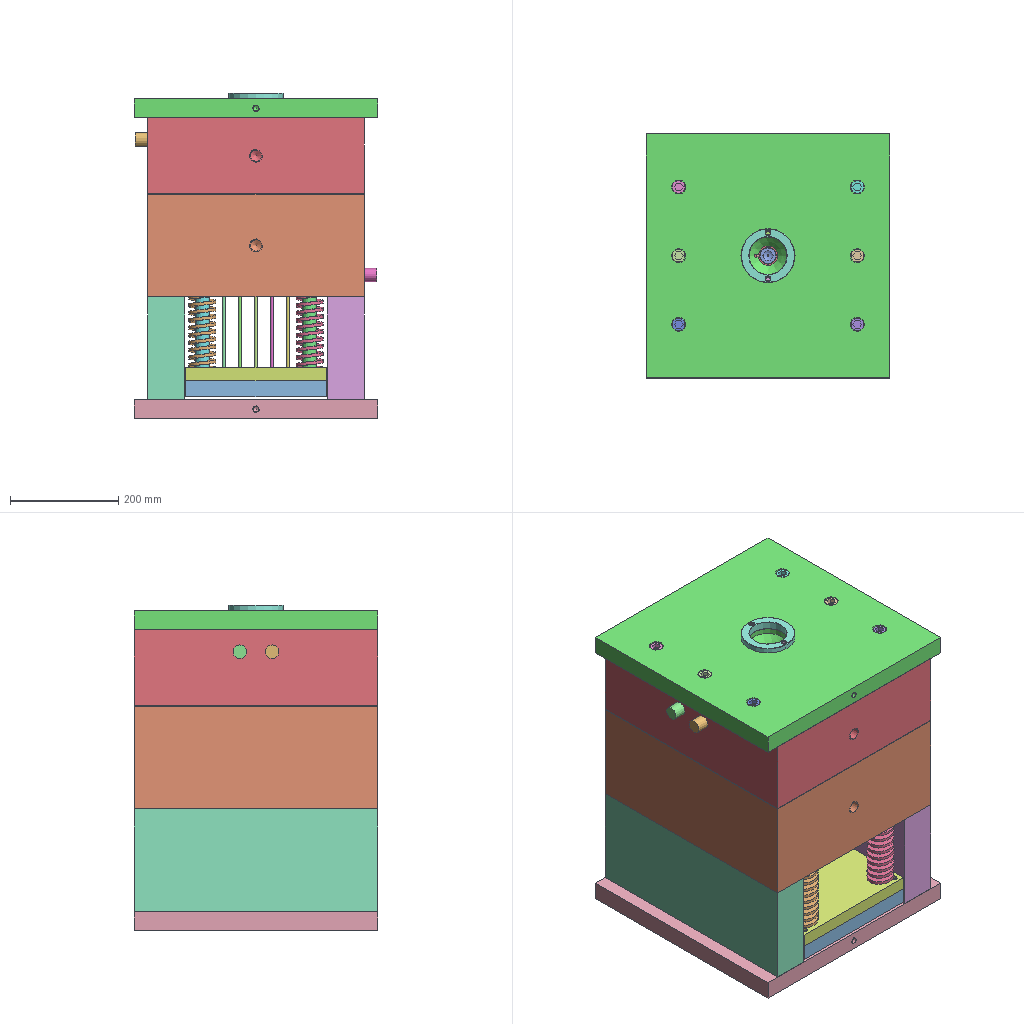Assembly | NX | 144 different items | 144 placed | box 450 x 450 x 601 mm
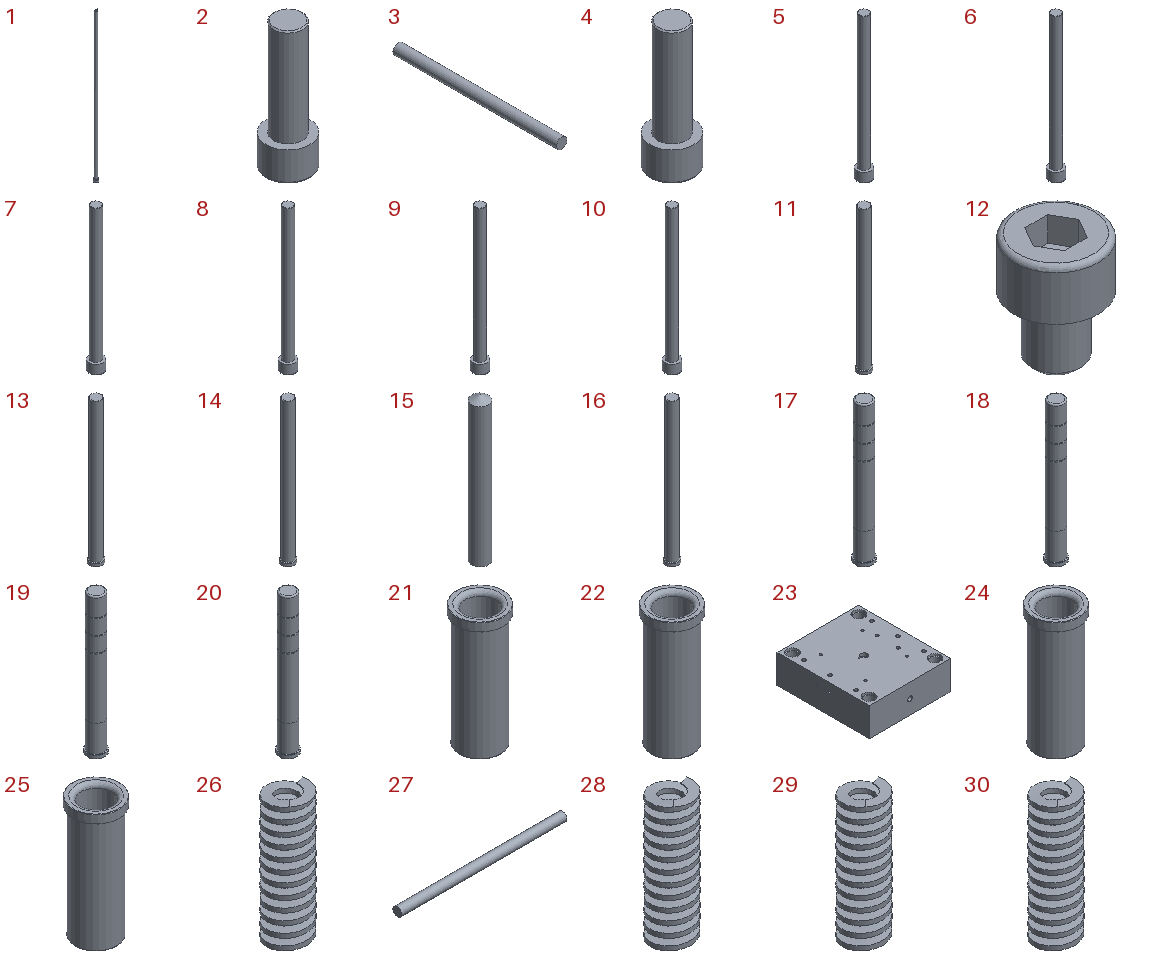Parts list (item | quantity | size | volume | features):
1 | x1 | 10 x 10 x 360.85 mm | 10434 mm3 | features solid 2
2 | x1 | 18 x 18 x 52 mm | 7050 mm3 | features solid 2
3 | x1 | 6 x 95.732 x 6 mm | 2674 mm3 | features solid 2
4 | x1 | 18 x 18 x 52 mm | 7050 mm3 | features solid 2
5 | x1 | 24 x 24 x 246 mm | 52114 mm3 | features solid 2
6 | x1 | 24 x 24 x 246 mm | 52114 mm3 | features solid 2
7 | x1 | 24 x 24 x 246 mm | 52114 mm3 | features solid 2
8 | x1 | 24 x 24 x 246 mm | 52114 mm3 | features solid 2
9 | x1 | 24 x 24 x 246 mm | 52114 mm3 | features solid 2
10 | x1 | 24 x 24 x 246 mm | 52114 mm3 | features solid 2
11 | x1 | 30 x 30 x 346 mm | 171537 mm3 | features solid 2
12 | x1 | 8.5 x 8.5 x 11 mm | 363.666 mm3 | features solid 2
13 | x1 | 30 x 30 x 346 mm | 171537 mm3 | features solid 2
14 | x1 | 30 x 30 x 346 mm | 171537 mm3 | features solid 2
15 | x1 | 6 x 6 x 50.732 mm | 1402 mm3 | features solid 2
16 | x1 | 30 x 30 x 346 mm | 171537 mm3 | features solid 2
17 | x1 | 40 x 40 x 320 mm | 309816 mm3 | features solid 2
18 | x1 | 40 x 40 x 320 mm | 309816 mm3 | features solid 2
19 | x1 | 40 x 40 x 320 mm | 309816 mm3 | features solid 2
20 | x1 | 40 x 40 x 320 mm | 309816 mm3 | features solid 2
21 | x1 | 54 x 54 x 140 mm | 122133 mm3 | features solid 2
22 | x1 | 54 x 54 x 140 mm | 122133 mm3 | features solid 2
23 | x1 | 400 x 450 x 140 mm | 19391135 mm3 | features solid 2
24 | x1 | 54 x 54 x 140 mm | 122133 mm3 | features solid 2
25 | x1 | 54 x 54 x 140 mm | 122133 mm3 | features solid 2
26 | x1 | 50.009 x 50.008 x 160 mm | 82264 mm3 | features solid 2
27 | x1 | 115 x 6 x 6 mm | 3252 mm3 | features solid 2
28 | x1 | 50.009 x 50.008 x 160 mm | 82264 mm3 | features solid 2
29 | x1 | 50.009 x 50.008 x 160 mm | 82264 mm3 | features solid 2
30 | x1 | 50.009 x 50.008 x 160 mm | 82264 mm3 | features solid 2
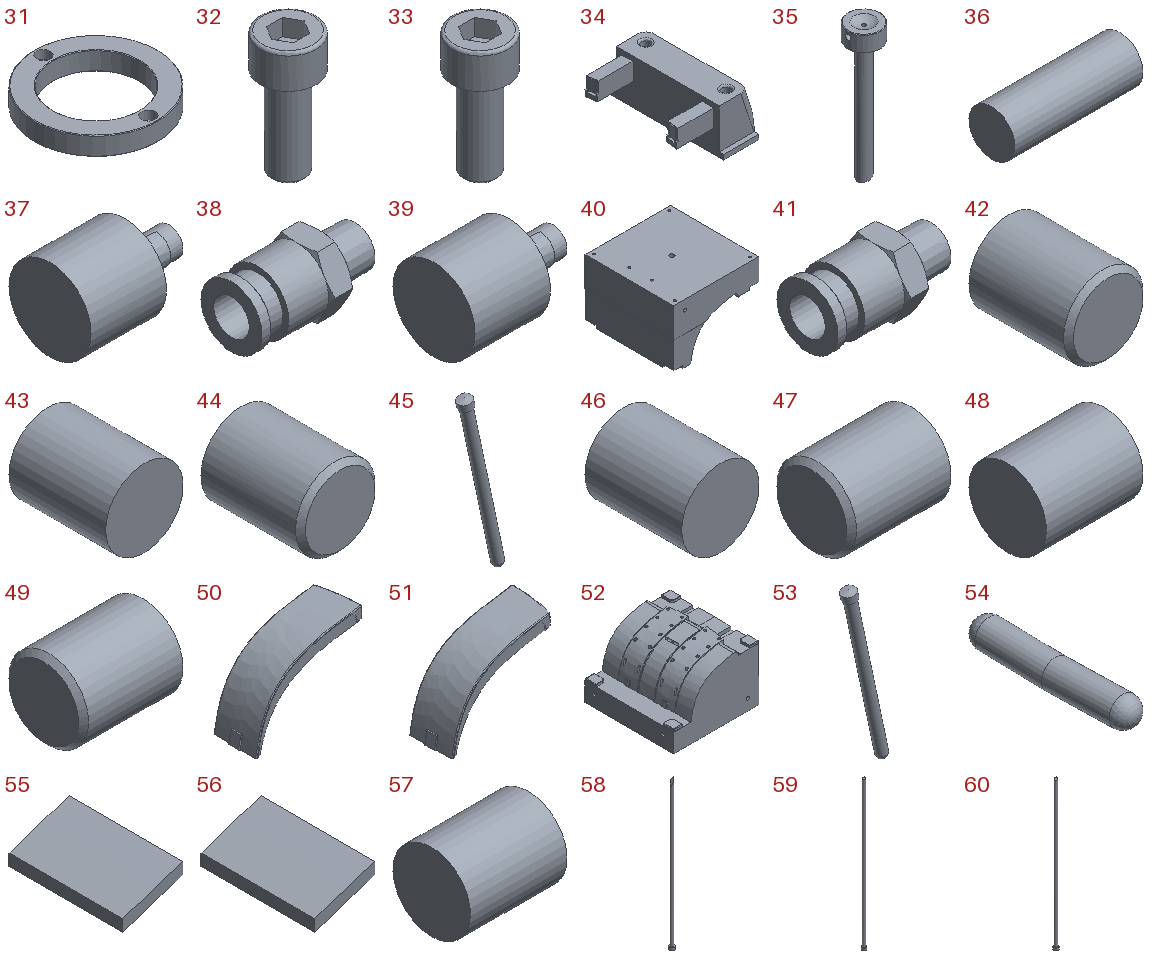31 | x1 | 99.8 x 99.8 x 15 mm | 57533 mm3 | features solid 2
32 | x1 | 10 x 10 x 22 mm | 854.803 mm3 | features solid 2
33 | x1 | 10 x 10 x 22 mm | 854.803 mm3 | features solid 2
34 | x1 | 92.291 x 144 x 57 mm | 348793 mm3 | features solid 2
35 | x1 | 30 x 30 x 126.717 mm | 19254 mm3 | features solid 2
36 | x1 | 14 x 5 x 5 mm | 274.889 mm3 | features solid 2
37 | x1 | 38.754 x 25 x 25 mm | 12122 mm3 | features solid 2
38 | x1 | 27.9 x 16.166 x 14 mm | 2279 mm3 | features solid 2
39 | x1 | 38.754 x 25 x 25 mm | 12122 mm3 | features solid 2
40 | x1 | 230 x 240 x 159.117 mm | 4798868 mm3 | features solid 2
41 | x1 | 27.9 x 16.166 x 14 mm | 2279 mm3 | features solid 2
42 | x1 | 8 x 10 x 8 mm | 499.644 mm3 | features solid 2
43 | x1 | 8 x 10 x 8 mm | 502.655 mm3 | features solid 2
44 | x1 | 8 x 10 x 8 mm | 499.644 mm3 | features solid 2
45 | x1 | 44.588 x 13 x 162.687 mm | 13234 mm3 | features solid 2
46 | x1 | 8 x 10 x 8 mm | 502.655 mm3 | features solid 2
47 | x1 | 10 x 8 x 8 mm | 499.644 mm3 | features solid 2
48 | x1 | 10 x 8 x 8 mm | 502.655 mm3 | features solid 2
49 | x1 | 10 x 8 x 8 mm | 499.644 mm3 | features solid 2
50 | x1 | 146.551 x 59 x 110.019 mm | 28651 mm3 | features Body 2
51 | x1 | 146.551 x 59 x 110.019 mm | 28651 mm3 | features Body 2
52 | x1 | 230 x 240 x 159.014 mm | 6548136 mm3 | features solid 2
53 | x1 | 44.588 x 13 x 162.687 mm | 13234 mm3 | features solid 2
54 | x1 | 6.099 x 34.468 x 6.24 mm | 918.133 mm3 | features solid 2
55 | x1 | 4 x 7.555 x 2.069 mm | 23.453 mm3 | features solid 2
56 | x1 | 4 x 7.555 x 2.069 mm | 23.453 mm3 | features solid 2
57 | x1 | 10 x 8 x 8 mm | 502.655 mm3 | features solid 2
58 | x1 | 10 x 10 x 315.042 mm | 9023 mm3 | features solid 2
59 | x1 | 10 x 10 x 362.073 mm | 10509 mm3 | features solid 2
60 | x1 | 10 x 10 x 348.483 mm | 10095 mm3 | features solid 2
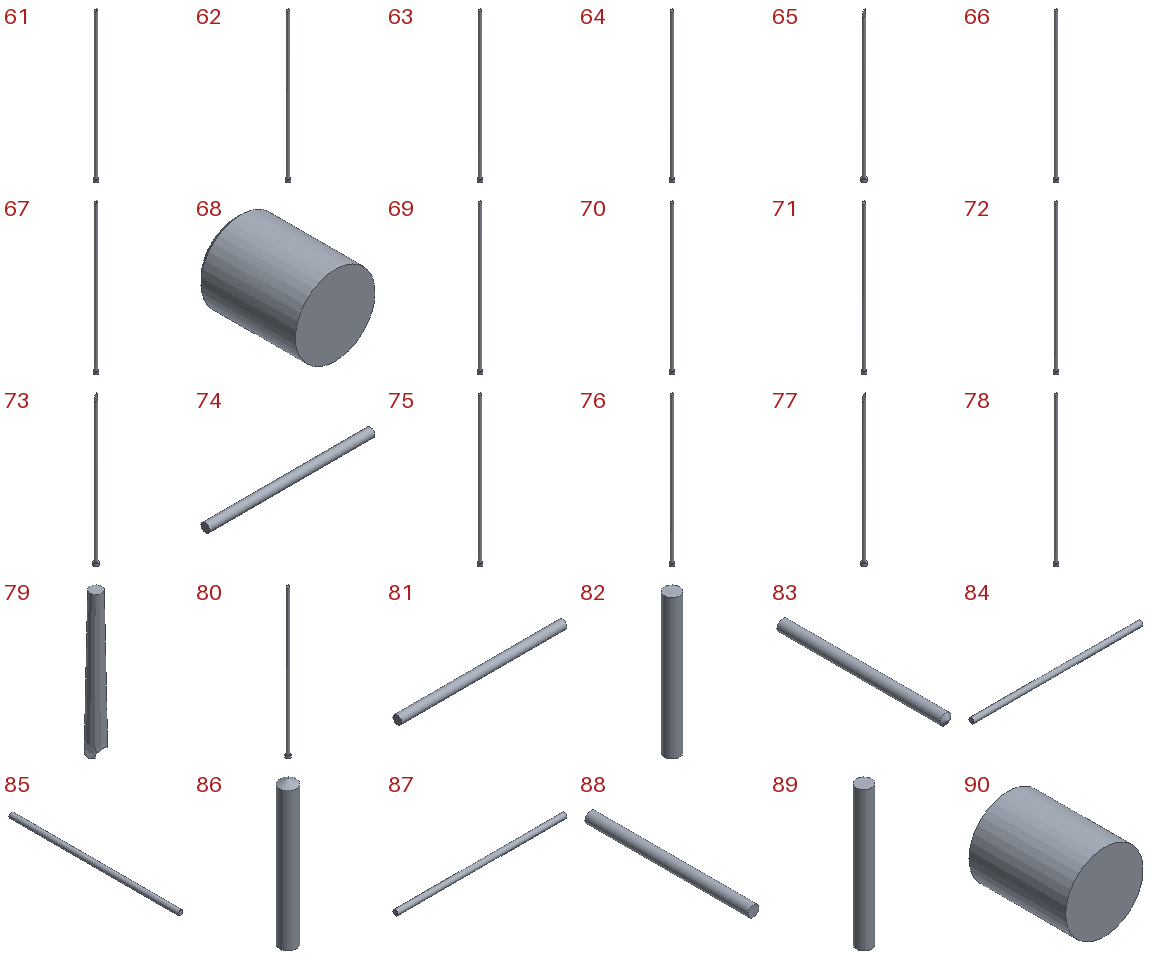61 | x1 | 10 x 10 x 372.984 mm | 10833 mm3 | features solid 2
62 | x1 | 10 x 10 x 368.654 mm | 10708 mm3 | features solid 2
63 | x1 | 10 x 10 x 362.708 mm | 10527 mm3 | features solid 2
64 | x1 | 10 x 10 x 349.469 mm | 10125 mm3 | features solid 2
65 | x1 | 10 x 10 x 317.079 mm | 9086 mm3 | features solid 2
66 | x1 | 10 x 10 x 369.226 mm | 10724 mm3 | features solid 2
67 | x1 | 10 x 10 x 373.555 mm | 10849 mm3 | features solid 2
68 | x1 | 8 x 10 x 8 mm | 499.644 mm3 | features solid 2
69 | x1 | 10 x 10 x 368.654 mm | 10708 mm3 | features solid 2
70 | x1 | 10 x 10 x 362.073 mm | 10509 mm3 | features solid 2
71 | x1 | 10 x 10 x 349.469 mm | 10124 mm3 | features solid 2
72 | x1 | 10 x 10 x 369.222 mm | 10724 mm3 | features solid 2
73 | x1 | 10 x 10 x 315.047 mm | 9022 mm3 | features solid 2
74 | x1 | 115 x 6 x 6 mm | 3252 mm3 | features solid 2
75 | x1 | 10 x 10 x 362.709 mm | 10527 mm3 | features solid 2
76 | x1 | 10 x 10 x 372.984 mm | 10833 mm3 | features solid 2
77 | x1 | 10 x 10 x 317.08 mm | 9086 mm3 | features solid 2
78 | x1 | 10 x 10 x 373.555 mm | 10849 mm3 | features solid 2
79 | x1 | 7.748 x 7.655 x 65.449 mm | 2152 mm3 | features solid 2
80 | x1 | 10 x 10 x 348.483 mm | 10094 mm3 | features solid 2
81 | x1 | 115 x 6 x 6 mm | 3252 mm3 | features solid 2
82 | x1 | 6 x 6 x 55.732 mm | 1543 mm3 | features solid 2
83 | x1 | 6 x 90.732 x 6 mm | 2533 mm3 | features solid 2
84 | x1 | 200 x 6 x 6 mm | 5655 mm3 | features solid 2
85 | x1 | 6 x 210 x 6 mm | 5938 mm3 | features solid 2
86 | x1 | 6 x 6 x 50.732 mm | 1402 mm3 | features solid 2
87 | x1 | 200 x 6 x 6 mm | 5655 mm3 | features solid 2
88 | x1 | 6 x 90.732 x 6 mm | 2533 mm3 | features solid 2
89 | x1 | 6 x 6 x 55.732 mm | 1543 mm3 | features solid 2
90 | x1 | 8 x 10 x 8 mm | 502.655 mm3 | features solid 2
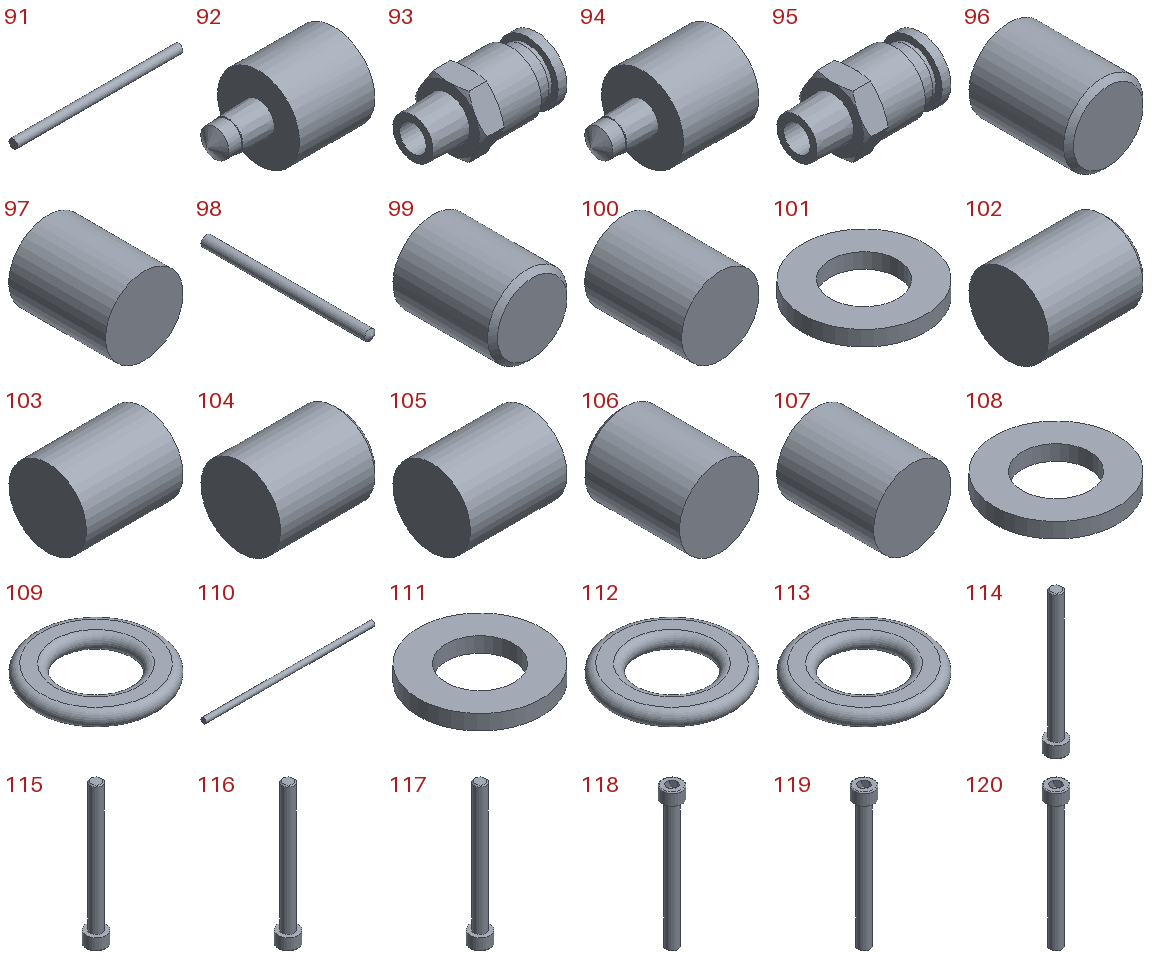91 | x1 | 115 x 6 x 6 mm | 3252 mm3 | features solid 2
92 | x1 | 38.754 x 25 x 25 mm | 12122 mm3 | features solid 2
93 | x1 | 27.9 x 16.166 x 14 mm | 2279 mm3 | features solid 2
94 | x1 | 38.754 x 25 x 25 mm | 12122 mm3 | features solid 2
95 | x1 | 27.9 x 16.166 x 14 mm | 2279 mm3 | features solid 2
96 | x1 | 8 x 10 x 8 mm | 499.644 mm3 | features solid 2
97 | x1 | 8 x 10 x 8 mm | 502.655 mm3 | features solid 2
98 | x1 | 6 x 95.732 x 6 mm | 2674 mm3 | features solid 2
99 | x1 | 8 x 10 x 8 mm | 499.644 mm3 | features solid 2
100 | x1 | 8 x 10 x 8 mm | 502.655 mm3 | features solid 2
101 | x1 | 14.6 x 14.6 x 1.8 mm | 210.87 mm3 | features solid 2
102 | x1 | 10 x 8 x 8 mm | 499.644 mm3 | features solid 2
103 | x1 | 10 x 8 x 8 mm | 502.655 mm3 | features solid 2
104 | x1 | 10 x 8 x 8 mm | 499.644 mm3 | features solid 2
105 | x1 | 10 x 8 x 8 mm | 502.655 mm3 | features solid 2
106 | x1 | 8 x 10 x 8 mm | 499.644 mm3 | features solid 2
107 | x1 | 8 x 10 x 8 mm | 502.655 mm3 | features solid 2
108 | x1 | 14.6 x 14.6 x 1.8 mm | 210.87 mm3 | features solid 2
109 | x1 | 14.6 x 14.6 x 1.8 mm | 186.186 mm3 | features solid 2
110 | x1 | 200 x 6 x 6 mm | 5655 mm3 | features solid 2
111 | x1 | 14.6 x 14.6 x 1.8 mm | 210.87 mm3 | features solid 2
112 | x1 | 14.6 x 14.6 x 1.8 mm | 186.186 mm3 | features solid 2
113 | x1 | 14.6 x 14.6 x 1.8 mm | 186.186 mm3 | features solid 2
114 | x1 | 10 x 10 x 71 mm | 2240 mm3 | features solid 2
115 | x1 | 10 x 10 x 71 mm | 2240 mm3 | features solid 2
116 | x1 | 10 x 10 x 71 mm | 2240 mm3 | features solid 2
117 | x1 | 10 x 10 x 71 mm | 2240 mm3 | features solid 2
118 | x1 | 10 x 10 x 71 mm | 2240 mm3 | features solid 2
119 | x1 | 10 x 10 x 71 mm | 2240 mm3 | features solid 2
120 | x1 | 10 x 10 x 71 mm | 2240 mm3 | features solid 2
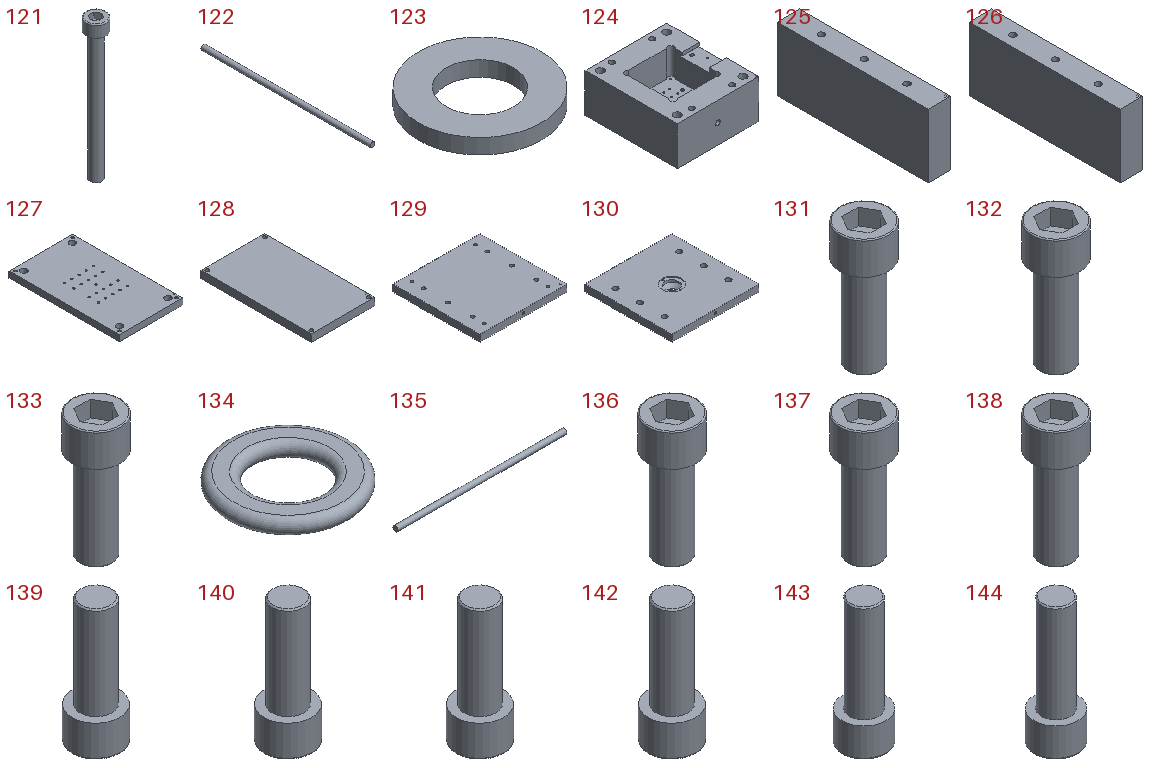121 | x1 | 10 x 10 x 71 mm | 2240 mm3 | features solid 2
122 | x1 | 6 x 210 x 6 mm | 5938 mm3 | features solid 2
123 | x1 | 14.6 x 14.6 x 1.8 mm | 210.87 mm3 | features solid 2
124 | x1 | 400 x 450 x 190 mm | 25227574 mm3 | features solid 2
125 | x1 | 68 x 450 x 190 mm | 5663632 mm3 | features solid 2
126 | x1 | 68 x 450 x 190 mm | 5663632 mm3 | features solid 2
127 | x1 | 260 x 450 x 25 mm | 2831486 mm3 | features solid 2
128 | x1 | 260 x 450 x 30 mm | 3483194 mm3 | features solid 2
129 | x1 | 450 x 450 x 35 mm | 6967341 mm3 | features solid 2
130 | x1 | 450 x 450 x 35 mm | 6878672 mm3 | features solid 2
131 | x1 | 24 x 24 x 61 mm | 14918 mm3 | features solid 2
132 | x1 | 24 x 24 x 61 mm | 14918 mm3 | features solid 2
133 | x1 | 24 x 24 x 61 mm | 14918 mm3 | features solid 2
134 | x1 | 14.6 x 14.6 x 1.8 mm | 186.186 mm3 | features solid 2
135 | x1 | 200 x 6 x 6 mm | 5655 mm3 | features solid 2
136 | x1 | 24 x 24 x 61 mm | 14918 mm3 | features solid 2
137 | x1 | 24 x 24 x 61 mm | 14918 mm3 | features solid 2
138 | x1 | 24 x 24 x 61 mm | 14918 mm3 | features solid 2
139 | x1 | 18 x 18 x 47 mm | 6485 mm3 | features solid 2
140 | x1 | 18 x 18 x 47 mm | 6485 mm3 | features solid 2
141 | x1 | 18 x 18 x 47 mm | 6485 mm3 | features solid 2
142 | x1 | 18 x 18 x 47 mm | 6485 mm3 | features solid 2
143 | x1 | 18 x 18 x 52 mm | 7050 mm3 | features solid 2
144 | x1 | 18 x 18 x 52 mm | 7050 mm3 | features solid 2